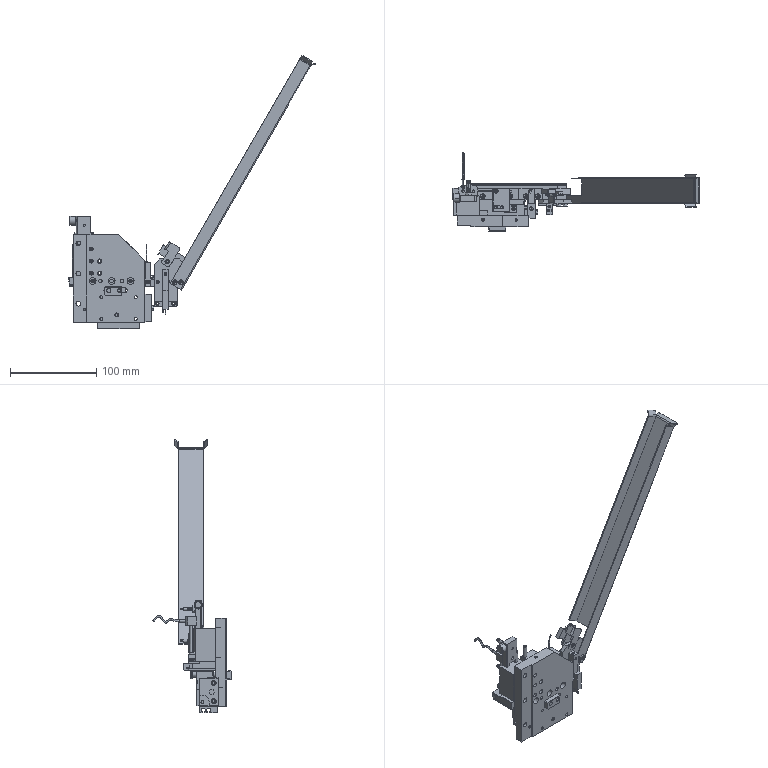Part | NX | 54 solids | 2619 faces | box 285.673 x 90.618 x 317.186 mm | volume 250392 mm3 | plane 1734 | cylinder 596 | cone 257 | spline 18 | torus 13 | sphere 1 | commonest cylinder face diameters 2.5 x99 4 x90 3 x56 3.3 x46 6 x30 5 x28